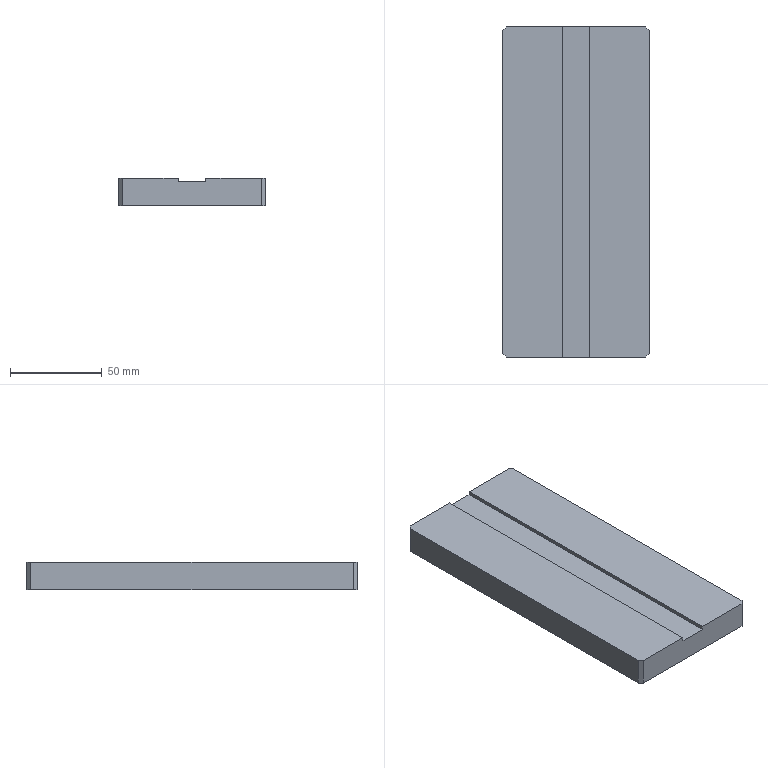Part | STEP file | Planar support platform base | 1 solid | 14 faces | box 80 x 180 x 15 mm | volume 210480 mm3 | plane 14
STEP:
#1=CARTESIAN_POINT('',(0.,0.,0.));
#2=DIRECTION('',(0.,0.,1.));
#3=DIRECTION('',(1.,0.,0.));
#4=AXIS2_PLACEMENT_3D('',#1,#2,#3);
#5=CARTESIAN_POINT('',(38.,90.,15.));
#6=VERTEX_POINT('',#5);
#7=CARTESIAN_POINT('',(7.5,90.,15.));
#8=VERTEX_POINT('',#7);
#9=CARTESIAN_POINT('',(-40.,90.,15.));
#10=DIRECTION('',(-1.,0.,0.));
#11=VECTOR('',#10,1.);
#12=LINE('',#9,#11);
#13=CARTESIAN_POINT('',(0.,0.,15.));
#14=DIRECTION('',(0.,0.,-1.));
#15=DIRECTION('',(-1.,0.,0.));
#16=AXIS2_PLACEMENT_3D('',#13,#14,#15);
#17=PLANE('',#16);
#18=CARTESIAN_POINT('',(40.,90.));
#19=DIRECTION('',(1.,0.));
#20=VECTOR('',#19,1.);
#21=LINE('',#18,#20);
#22=(GEOMETRIC_REPRESENTATION_CONTEXT(2)PARAMETRIC_REPRESENTATION_CONTEXT()REPRESENTATION_CONTEXT('',''));
#23=DEFINITIONAL_REPRESENTATION('',(#21),#22);
#24=PCURVE('',#17,#23);
#25=CARTESIAN_POINT('',(-40.,90.,15.));
#26=DIRECTION('',(0.,-1.,0.));
#27=DIRECTION('',(1.,0.,0.));
#28=AXIS2_PLACEMENT_3D('',#25,#26,#27);
#29=PLANE('',#28);
#30=CARTESIAN_POINT('',(0.,0.));
#31=DIRECTION('',(-1.,0.));
#32=VECTOR('',#31,1.);
#33=LINE('',#30,#32);
#34=(GEOMETRIC_REPRESENTATION_CONTEXT(2)PARAMETRIC_REPRESENTATION_CONTEXT()REPRESENTATION_CONTEXT('',''));
#35=DEFINITIONAL_REPRESENTATION('',(#33),#34);
#36=PCURVE('',#29,#35);
#37=SURFACE_CURVE('',#12,(#24,#36),.PCURVE_S1.);
#38=EDGE_CURVE('',#6,#8,#37,.T.);
#39=ORIENTED_EDGE('',*,*,#38,.T.);
#40=CARTESIAN_POINT('',(7.5,-90.,15.));
#41=VERTEX_POINT('',#40);
#42=CARTESIAN_POINT('',(7.5,-90.,15.));
#43=DIRECTION('',(0.,1.,0.));
#44=VECTOR('',#43,1.);
#45=LINE('',#42,#44);
#46=CARTESIAN_POINT('',(-7.5,-90.));
#47=DIRECTION('',(0.,1.));
#48=VECTOR('',#47,1.);
#49=LINE('',#46,#48);
#50=(GEOMETRIC_REPRESENTATION_CONTEXT(2)PARAMETRIC_REPRESENTATION_CONTEXT()REPRESENTATION_CONTEXT('',''));
#51=DEFINITIONAL_REPRESENTATION('',(#49),#50);
#52=PCURVE('',#17,#51);
#53=CARTESIAN_POINT('',(7.5,-90.,15.));
#54=DIRECTION('',(1.,0.,0.));
#55=DIRECTION('',(0.,0.,-1.));
#56=AXIS2_PLACEMENT_3D('',#53,#54,#55);
#57=PLANE('',#56);
#58=CARTESIAN_POINT('',(0.,0.));
#59=DIRECTION('',(0.,1.));
#60=VECTOR('',#59,1.);
#61=LINE('',#58,#60);
#62=(GEOMETRIC_REPRESENTATION_CONTEXT(2)PARAMETRIC_REPRESENTATION_CONTEXT()REPRESENTATION_CONTEXT('',''));
#63=DEFINITIONAL_REPRESENTATION('',(#61),#62);
#64=PCURVE('',#57,#63);
#65=SURFACE_CURVE('',#45,(#52,#64),.PCURVE_S1.);
#66=EDGE_CURVE('',#41,#8,#65,.T.);
#67=ORIENTED_EDGE('',*,*,#66,.F.);
#68=CARTESIAN_POINT('',(38.,-90.,15.));
#69=VERTEX_POINT('',#68);
#70=CARTESIAN_POINT('',(-40.,-90.,15.));
#71=DIRECTION('',(1.,0.,0.));
#72=VECTOR('',#71,1.);
#73=LINE('',#70,#72);
#74=CARTESIAN_POINT('',(40.,-90.));
#75=DIRECTION('',(-1.,0.));
#76=VECTOR('',#75,1.);
#77=LINE('',#74,#76);
#78=(GEOMETRIC_REPRESENTATION_CONTEXT(2)PARAMETRIC_REPRESENTATION_CONTEXT()REPRESENTATION_CONTEXT('',''));
#79=DEFINITIONAL_REPRESENTATION('',(#77),#78);
#80=PCURVE('',#17,#79);
#81=CARTESIAN_POINT('',(-40.,-90.,15.));
#82=DIRECTION('',(0.,1.,0.));
#83=DIRECTION('',(-1.,0.,0.));
#84=AXIS2_PLACEMENT_3D('',#81,#82,#83);
#85=PLANE('',#84);
#86=CARTESIAN_POINT('',(0.,0.));
#87=DIRECTION('',(-1.,0.));
#88=VECTOR('',#87,1.);
#89=LINE('',#86,#88);
#90=(GEOMETRIC_REPRESENTATION_CONTEXT(2)PARAMETRIC_REPRESENTATION_CONTEXT()REPRESENTATION_CONTEXT('',''));
#91=DEFINITIONAL_REPRESENTATION('',(#89),#90);
#92=PCURVE('',#85,#91);
#93=SURFACE_CURVE('',#73,(#80,#92),.PCURVE_S1.);
#94=EDGE_CURVE('',#41,#69,#93,.T.);
#95=ORIENTED_EDGE('',*,*,#94,.T.);
#96=CARTESIAN_POINT('',(40.,-88.,15.));
#97=VERTEX_POINT('',#96);
#98=CARTESIAN_POINT('',(40.,-88.,15.));
#99=DIRECTION('',(0.7071,0.7071,0.));
#100=VECTOR('',#99,1.);
#101=LINE('',#98,#100);
#102=CARTESIAN_POINT('',(-40.,-88.));
#103=DIRECTION('',(-0.7071,0.7071));
#104=VECTOR('',#103,1.);
#105=LINE('',#102,#104);
#106=(GEOMETRIC_REPRESENTATION_CONTEXT(2)PARAMETRIC_REPRESENTATION_CONTEXT()REPRESENTATION_CONTEXT('',''));
#107=DEFINITIONAL_REPRESENTATION('',(#105),#106);
#108=PCURVE('',#17,#107);
#109=CARTESIAN_POINT('',(40.,-88.,15.));
#110=DIRECTION('',(-0.7071,0.7071,0.));
#111=DIRECTION('',(0.,0.,-1.));
#112=AXIS2_PLACEMENT_3D('',#109,#110,#111);
#113=PLANE('',#112);
#114=CARTESIAN_POINT('',(0.,0.));
#115=DIRECTION('',(0.,-1.));
#116=VECTOR('',#115,1.);
#117=LINE('',#114,#116);
#118=(GEOMETRIC_REPRESENTATION_CONTEXT(2)PARAMETRIC_REPRESENTATION_CONTEXT()REPRESENTATION_CONTEXT('',''));
#119=DEFINITIONAL_REPRESENTATION('',(#117),#118);
#120=PCURVE('',#113,#119);
#121=SURFACE_CURVE('',#101,(#108,#120),.PCURVE_S1.);
#122=EDGE_CURVE('',#69,#97,#121,.T.);
#123=ORIENTED_EDGE('',*,*,#122,.T.);
#124=CARTESIAN_POINT('',(40.,88.,15.));
#125=VERTEX_POINT('',#124);
#126=CARTESIAN_POINT('',(40.,-90.,15.));
#127=DIRECTION('',(0.,1.,0.));
#128=VECTOR('',#127,1.);
#129=LINE('',#126,#128);
#130=CARTESIAN_POINT('',(-40.,-90.));
#131=DIRECTION('',(0.,1.));
#132=VECTOR('',#131,1.);
#133=LINE('',#130,#132);
#134=(GEOMETRIC_REPRESENTATION_CONTEXT(2)PARAMETRIC_REPRESENTATION_CONTEXT()REPRESENTATION_CONTEXT('',''));
#135=DEFINITIONAL_REPRESENTATION('',(#133),#134);
#136=PCURVE('',#17,#135);
#137=CARTESIAN_POINT('',(40.,-90.,15.));
#138=DIRECTION('',(-1.,0.,0.));
#139=DIRECTION('',(0.,0.,1.));
#140=AXIS2_PLACEMENT_3D('',#137,#138,#139);
#141=PLANE('',#140);
#142=CARTESIAN_POINT('',(0.,0.));
#143=DIRECTION('',(0.,1.));
#144=VECTOR('',#143,1.);
#145=LINE('',#142,#144);
#146=(GEOMETRIC_REPRESENTATION_CONTEXT(2)PARAMETRIC_REPRESENTATION_CONTEXT()REPRESENTATION_CONTEXT('',''));
#147=DEFINITIONAL_REPRESENTATION('',(#145),#146);
#148=PCURVE('',#141,#147);
#149=SURFACE_CURVE('',#129,(#136,#148),.PCURVE_S1.);
#150=EDGE_CURVE('',#97,#125,#149,.T.);
#151=ORIENTED_EDGE('',*,*,#150,.T.);
#152=CARTESIAN_POINT('',(38.,90.,15.));
#153=DIRECTION('',(-0.7071,0.7071,0.));
#154=VECTOR('',#153,1.);
#155=LINE('',#152,#154);
#156=CARTESIAN_POINT('',(-38.,90.));
#157=DIRECTION('',(0.7071,0.7071));
#158=VECTOR('',#157,1.);
#159=LINE('',#156,#158);
#160=(GEOMETRIC_REPRESENTATION_CONTEXT(2)PARAMETRIC_REPRESENTATION_CONTEXT()REPRESENTATION_CONTEXT('',''));
#161=DEFINITIONAL_REPRESENTATION('',(#159),#160);
#162=PCURVE('',#17,#161);
#163=CARTESIAN_POINT('',(38.,90.,15.));
#164=DIRECTION('',(-0.7071,-0.7071,0.));
#165=DIRECTION('',(0.,0.,-1.));
#166=AXIS2_PLACEMENT_3D('',#163,#164,#165);
#167=PLANE('',#166);
#168=CARTESIAN_POINT('',(0.,0.));
#169=DIRECTION('',(0.,-1.));
#170=VECTOR('',#169,1.);
#171=LINE('',#168,#170);
#172=(GEOMETRIC_REPRESENTATION_CONTEXT(2)PARAMETRIC_REPRESENTATION_CONTEXT()REPRESENTATION_CONTEXT('',''));
#173=DEFINITIONAL_REPRESENTATION('',(#171),#172);
#174=PCURVE('',#167,#173);
#175=SURFACE_CURVE('',#155,(#162,#174),.PCURVE_S1.);
#176=EDGE_CURVE('',#125,#6,#175,.T.);
#177=ORIENTED_EDGE('',*,*,#176,.T.);
#178=EDGE_LOOP('',(#39,#67,#95,#123,#151,#177));
#179=FACE_BOUND('',#178,.T.);
#180=ADVANCED_FACE('',(#179),#17,.F.);
#181=ORIENTED_EDGE('',*,*,#150,.F.);
#182=CARTESIAN_POINT('',(40.,-88.,0.));
#183=VERTEX_POINT('',#182);
#184=CARTESIAN_POINT('',(40.,-88.,15.));
#185=DIRECTION('',(0.,0.,-1.));
#186=VECTOR('',#185,1.);
#187=LINE('',#184,#186);
#188=CARTESIAN_POINT('',(0.,2.));
#189=DIRECTION('',(-1.,0.));
#190=VECTOR('',#189,1.);
#191=LINE('',#188,#190);
#192=(GEOMETRIC_REPRESENTATION_CONTEXT(2)PARAMETRIC_REPRESENTATION_CONTEXT()REPRESENTATION_CONTEXT('',''));
#193=DEFINITIONAL_REPRESENTATION('',(#191),#192);
#194=PCURVE('',#141,#193);
#195=CARTESIAN_POINT('',(0.,0.));
#196=DIRECTION('',(1.,0.));
#197=VECTOR('',#196,1.);
#198=LINE('',#195,#197);
#199=(GEOMETRIC_REPRESENTATION_CONTEXT(2)PARAMETRIC_REPRESENTATION_CONTEXT()REPRESENTATION_CONTEXT('',''));
#200=DEFINITIONAL_REPRESENTATION('',(#198),#199);
#201=PCURVE('',#113,#200);
#202=SURFACE_CURVE('',#187,(#194,#201),.PCURVE_S1.);
#203=EDGE_CURVE('',#97,#183,#202,.T.);
#204=ORIENTED_EDGE('',*,*,#203,.T.);
#205=CARTESIAN_POINT('',(40.,88.,0.));
#206=VERTEX_POINT('',#205);
#207=CARTESIAN_POINT('',(40.,-90.,0.));
#208=DIRECTION('',(0.,1.,0.));
#209=VECTOR('',#208,1.);
#210=LINE('',#207,#209);
#211=CARTESIAN_POINT('',(-15.,0.));
#212=DIRECTION('',(0.,1.));
#213=VECTOR('',#212,1.);
#214=LINE('',#211,#213);
#215=(GEOMETRIC_REPRESENTATION_CONTEXT(2)PARAMETRIC_REPRESENTATION_CONTEXT()REPRESENTATION_CONTEXT('',''));
#216=DEFINITIONAL_REPRESENTATION('',(#214),#215);
#217=PCURVE('',#141,#216);
#218=CARTESIAN_POINT('',(0.,0.,0.));
#219=DIRECTION('',(0.,0.,-1.));
#220=DIRECTION('',(-1.,0.,0.));
#221=AXIS2_PLACEMENT_3D('',#218,#219,#220);
#222=PLANE('',#221);
#223=CARTESIAN_POINT('',(-40.,-90.));
#224=DIRECTION('',(0.,1.));
#225=VECTOR('',#224,1.);
#226=LINE('',#223,#225);
#227=(GEOMETRIC_REPRESENTATION_CONTEXT(2)PARAMETRIC_REPRESENTATION_CONTEXT()REPRESENTATION_CONTEXT('',''));
#228=DEFINITIONAL_REPRESENTATION('',(#226),#227);
#229=PCURVE('',#222,#228);
#230=SURFACE_CURVE('',#210,(#217,#229),.PCURVE_S1.);
#231=EDGE_CURVE('',#183,#206,#230,.T.);
#232=ORIENTED_EDGE('',*,*,#231,.T.);
#233=CARTESIAN_POINT('',(40.,88.,15.));
#234=DIRECTION('',(0.,0.,1.));
#235=VECTOR('',#234,1.);
#236=LINE('',#233,#235);
#237=CARTESIAN_POINT('',(0.,178.));
#238=DIRECTION('',(1.,0.));
#239=VECTOR('',#238,1.);
#240=LINE('',#237,#239);
#241=(GEOMETRIC_REPRESENTATION_CONTEXT(2)PARAMETRIC_REPRESENTATION_CONTEXT()REPRESENTATION_CONTEXT('',''));
#242=DEFINITIONAL_REPRESENTATION('',(#240),#241);
#243=PCURVE('',#141,#242);
#244=CARTESIAN_POINT('',(0.,2.828));
#245=DIRECTION('',(-1.,0.));
#246=VECTOR('',#245,1.);
#247=LINE('',#244,#246);
#248=(GEOMETRIC_REPRESENTATION_CONTEXT(2)PARAMETRIC_REPRESENTATION_CONTEXT()REPRESENTATION_CONTEXT('',''));
#249=DEFINITIONAL_REPRESENTATION('',(#247),#248);
#250=PCURVE('',#167,#249);
#251=SURFACE_CURVE('',#236,(#243,#250),.PCURVE_S1.);
#252=EDGE_CURVE('',#206,#125,#251,.T.);
#253=ORIENTED_EDGE('',*,*,#252,.T.);
#254=EDGE_LOOP('',(#181,#204,#232,#253));
#255=FACE_BOUND('',#254,.T.);
#256=ADVANCED_FACE('',(#255),#141,.F.);
#257=CARTESIAN_POINT('',(7.5,90.,13.));
#258=VERTEX_POINT('',#257);
#259=CARTESIAN_POINT('',(-7.5,90.,13.));
#260=VERTEX_POINT('',#259);
#261=CARTESIAN_POINT('',(7.5,90.,13.));
#262=DIRECTION('',(-1.,0.,0.));
#263=VECTOR('',#262,1.);
#264=LINE('',#261,#263);
#265=CARTESIAN_POINT('',(47.5,-2.));
#266=DIRECTION('',(-1.,0.));
#267=VECTOR('',#266,1.);
#268=LINE('',#265,#267);
#269=(GEOMETRIC_REPRESENTATION_CONTEXT(2)PARAMETRIC_REPRESENTATION_CONTEXT()REPRESENTATION_CONTEXT('',''));
#270=DEFINITIONAL_REPRESENTATION('',(#268),#269);
#271=PCURVE('',#29,#270);
#272=CARTESIAN_POINT('',(7.5,-90.,13.));
#273=DIRECTION('',(0.,0.,-1.));
#274=DIRECTION('',(-1.,0.,0.));
#275=AXIS2_PLACEMENT_3D('',#272,#273,#274);
#276=PLANE('',#275);
#277=CARTESIAN_POINT('',(0.,180.));
#278=DIRECTION('',(1.,0.));
#279=VECTOR('',#278,1.);
#280=LINE('',#277,#279);
#281=(GEOMETRIC_REPRESENTATION_CONTEXT(2)PARAMETRIC_REPRESENTATION_CONTEXT()REPRESENTATION_CONTEXT('',''));
#282=DEFINITIONAL_REPRESENTATION('',(#280),#281);
#283=PCURVE('',#276,#282);
#284=SURFACE_CURVE('',#264,(#271,#283),.PCURVE_S1.);
#285=EDGE_CURVE('',#258,#260,#284,.T.);
#286=ORIENTED_EDGE('',*,*,#285,.F.);
#287=CARTESIAN_POINT('',(7.5,90.,15.));
#288=DIRECTION('',(0.,0.,-1.));
#289=VECTOR('',#288,1.);
#290=LINE('',#287,#289);
#291=CARTESIAN_POINT('',(47.5,0.));
#292=DIRECTION('',(0.,-1.));
#293=VECTOR('',#292,1.);
#294=LINE('',#291,#293);
#295=(GEOMETRIC_REPRESENTATION_CONTEXT(2)PARAMETRIC_REPRESENTATION_CONTEXT()REPRESENTATION_CONTEXT('',''));
#296=DEFINITIONAL_REPRESENTATION('',(#294),#295);
#297=PCURVE('',#29,#296);
#298=CARTESIAN_POINT('',(0.,180.));
#299=DIRECTION('',(1.,0.));
#300=VECTOR('',#299,1.);
#301=LINE('',#298,#300);
#302=(GEOMETRIC_REPRESENTATION_CONTEXT(2)PARAMETRIC_REPRESENTATION_CONTEXT()REPRESENTATION_CONTEXT('',''));
#303=DEFINITIONAL_REPRESENTATION('',(#301),#302);
#304=PCURVE('',#57,#303);
#305=SURFACE_CURVE('',#290,(#297,#304),.PCURVE_S1.);
#306=EDGE_CURVE('',#8,#258,#305,.T.);
#307=ORIENTED_EDGE('',*,*,#306,.F.);
#308=ORIENTED_EDGE('',*,*,#38,.F.);
#309=CARTESIAN_POINT('',(38.,90.,0.));
#310=VERTEX_POINT('',#309);
#311=CARTESIAN_POINT('',(38.,90.,15.));
#312=DIRECTION('',(0.,0.,-1.));
#313=VECTOR('',#312,1.);
#314=LINE('',#311,#313);
#315=CARTESIAN_POINT('',(78.,0.));
#316=DIRECTION('',(0.,-1.));
#317=VECTOR('',#316,1.);
#318=LINE('',#315,#317);
#319=(GEOMETRIC_REPRESENTATION_CONTEXT(2)PARAMETRIC_REPRESENTATION_CONTEXT()REPRESENTATION_CONTEXT('',''));
#320=DEFINITIONAL_REPRESENTATION('',(#318),#319);
#321=PCURVE('',#29,#320);
#322=CARTESIAN_POINT('',(0.,0.));
#323=DIRECTION('',(1.,0.));
#324=VECTOR('',#323,1.);
#325=LINE('',#322,#324);
#326=(GEOMETRIC_REPRESENTATION_CONTEXT(2)PARAMETRIC_REPRESENTATION_CONTEXT()REPRESENTATION_CONTEXT('',''));
#327=DEFINITIONAL_REPRESENTATION('',(#325),#326);
#328=PCURVE('',#167,#327);
#329=SURFACE_CURVE('',#314,(#321,#328),.PCURVE_S1.);
#330=EDGE_CURVE('',#6,#310,#329,.T.);
#331=ORIENTED_EDGE('',*,*,#330,.T.);
#332=CARTESIAN_POINT('',(-38.,90.,0.));
#333=VERTEX_POINT('',#332);
#334=CARTESIAN_POINT('',(-40.,90.,0.));
#335=DIRECTION('',(-1.,0.,0.));
#336=VECTOR('',#335,1.);
#337=LINE('',#334,#336);
#338=CARTESIAN_POINT('',(0.,-15.));
#339=DIRECTION('',(-1.,0.));
#340=VECTOR('',#339,1.);
#341=LINE('',#338,#340);
#342=(GEOMETRIC_REPRESENTATION_CONTEXT(2)PARAMETRIC_REPRESENTATION_CONTEXT()REPRESENTATION_CONTEXT('',''));
#343=DEFINITIONAL_REPRESENTATION('',(#341),#342);
#344=PCURVE('',#29,#343);
#345=CARTESIAN_POINT('',(40.,90.));
#346=DIRECTION('',(1.,0.));
#347=VECTOR('',#346,1.);
#348=LINE('',#345,#347);
#349=(GEOMETRIC_REPRESENTATION_CONTEXT(2)PARAMETRIC_REPRESENTATION_CONTEXT()REPRESENTATION_CONTEXT('',''));
#350=DEFINITIONAL_REPRESENTATION('',(#348),#349);
#351=PCURVE('',#222,#350);
#352=SURFACE_CURVE('',#337,(#344,#351),.PCURVE_S1.);
#353=EDGE_CURVE('',#310,#333,#352,.T.);
#354=ORIENTED_EDGE('',*,*,#353,.T.);
#355=CARTESIAN_POINT('',(-38.,90.,15.));
#356=VERTEX_POINT('',#355);
#357=CARTESIAN_POINT('',(-38.,90.,15.));
#358=DIRECTION('',(0.,0.,1.));
#359=VECTOR('',#358,1.);
#360=LINE('',#357,#359);
#361=CARTESIAN_POINT('',(2.,0.));
#362=DIRECTION('',(0.,1.));
#363=VECTOR('',#362,1.);
#364=LINE('',#361,#363);
#365=(GEOMETRIC_REPRESENTATION_CONTEXT(2)PARAMETRIC_REPRESENTATION_CONTEXT()REPRESENTATION_CONTEXT('',''));
#366=DEFINITIONAL_REPRESENTATION('',(#364),#365);
#367=PCURVE('',#29,#366);
#368=CARTESIAN_POINT('',(-40.,88.,15.));
#369=DIRECTION('',(0.7071,-0.7071,0.));
#370=DIRECTION('',(0.,0.,-1.));
#371=AXIS2_PLACEMENT_3D('',#368,#369,#370);
#372=PLANE('',#371);
#373=CARTESIAN_POINT('',(0.,2.828));
#374=DIRECTION('',(-1.,0.));
#375=VECTOR('',#374,1.);
#376=LINE('',#373,#375);
#377=(GEOMETRIC_REPRESENTATION_CONTEXT(2)PARAMETRIC_REPRESENTATION_CONTEXT()REPRESENTATION_CONTEXT('',''));
#378=DEFINITIONAL_REPRESENTATION('',(#376),#377);
#379=PCURVE('',#372,#378);
#380=SURFACE_CURVE('',#360,(#367,#379),.PCURVE_S1.);
#381=EDGE_CURVE('',#333,#356,#380,.T.);
#382=ORIENTED_EDGE('',*,*,#381,.T.);
#383=CARTESIAN_POINT('',(-7.5,90.,15.));
#384=VERTEX_POINT('',#383);
#385=CARTESIAN_POINT('',(-40.,90.,15.));
#386=DIRECTION('',(-1.,0.,0.));
#387=VECTOR('',#386,1.);
#388=LINE('',#385,#387);
#389=CARTESIAN_POINT('',(0.,0.));
#390=DIRECTION('',(-1.,0.));
#391=VECTOR('',#390,1.);
#392=LINE('',#389,#391);
#393=(GEOMETRIC_REPRESENTATION_CONTEXT(2)PARAMETRIC_REPRESENTATION_CONTEXT()REPRESENTATION_CONTEXT('',''));
#394=DEFINITIONAL_REPRESENTATION('',(#392),#393);
#395=PCURVE('',#29,#394);
#396=CARTESIAN_POINT('',(0.,0.,15.));
#397=DIRECTION('',(0.,0.,-1.));
#398=DIRECTION('',(-1.,0.,0.));
#399=AXIS2_PLACEMENT_3D('',#396,#397,#398);
#400=PLANE('',#399);
#401=CARTESIAN_POINT('',(40.,90.));
#402=DIRECTION('',(1.,0.));
#403=VECTOR('',#402,1.);
#404=LINE('',#401,#403);
#405=(GEOMETRIC_REPRESENTATION_CONTEXT(2)PARAMETRIC_REPRESENTATION_CONTEXT()REPRESENTATION_CONTEXT('',''));
#406=DEFINITIONAL_REPRESENTATION('',(#404),#405);
#407=PCURVE('',#400,#406);
#408=SURFACE_CURVE('',#388,(#395,#407),.PCURVE_S1.);
#409=EDGE_CURVE('',#384,#356,#408,.T.);
#410=ORIENTED_EDGE('',*,*,#409,.F.);
#411=CARTESIAN_POINT('',(-7.5,90.,15.));
#412=DIRECTION('',(0.,0.,1.));
#413=VECTOR('',#412,1.);
#414=LINE('',#411,#413);
#415=CARTESIAN_POINT('',(32.5,0.));
#416=DIRECTION('',(0.,1.));
#417=VECTOR('',#416,1.);
#418=LINE('',#415,#417);
#419=(GEOMETRIC_REPRESENTATION_CONTEXT(2)PARAMETRIC_REPRESENTATION_CONTEXT()REPRESENTATION_CONTEXT('',''));
#420=DEFINITIONAL_REPRESENTATION('',(#418),#419);
#421=PCURVE('',#29,#420);
#422=CARTESIAN_POINT('',(-7.5,-90.,15.));
#423=DIRECTION('',(-1.,0.,0.));
#424=DIRECTION('',(0.,-1.,0.));
#425=AXIS2_PLACEMENT_3D('',#422,#423,#424);
#426=PLANE('',#425);
#427=CARTESIAN_POINT('',(-180.,0.));
#428=DIRECTION('',(0.,1.));
#429=VECTOR('',#428,1.);
#430=LINE('',#427,#429);
#431=(GEOMETRIC_REPRESENTATION_CONTEXT(2)PARAMETRIC_REPRESENTATION_CONTEXT()REPRESENTATION_CONTEXT('',''));
#432=DEFINITIONAL_REPRESENTATION('',(#430),#431);
#433=PCURVE('',#426,#432);
#434=SURFACE_CURVE('',#414,(#421,#433),.PCURVE_S1.);
#435=EDGE_CURVE('',#260,#384,#434,.T.);
#436=ORIENTED_EDGE('',*,*,#435,.F.);
#437=EDGE_LOOP('',(#286,#307,#308,#331,#354,#382,#410,#436));
#438=FACE_BOUND('',#437,.T.);
#439=ADVANCED_FACE('',(#438),#29,.F.);
#440=CARTESIAN_POINT('',(-40.,88.,0.));
#441=VERTEX_POINT('',#440);
#442=CARTESIAN_POINT('',(-40.,-88.,0.));
#443=VERTEX_POINT('',#442);
#444=CARTESIAN_POINT('',(-40.,-90.,0.));
#445=DIRECTION('',(0.,-1.,0.));
#446=VECTOR('',#445,1.);
#447=LINE('',#444,#446);
#448=CARTESIAN_POINT('',(-40.,-90.,15.));
#449=DIRECTION('',(1.,0.,0.));
#450=DIRECTION('',(0.,1.,0.));
#451=AXIS2_PLACEMENT_3D('',#448,#449,#450);
#452=PLANE('',#451);
#453=CARTESIAN_POINT('',(0.,-15.));
#454=DIRECTION('',(-1.,0.));
#455=VECTOR('',#454,1.);
#456=LINE('',#453,#455);
#457=(GEOMETRIC_REPRESENTATION_CONTEXT(2)PARAMETRIC_REPRESENTATION_CONTEXT()REPRESENTATION_CONTEXT('',''));
#458=DEFINITIONAL_REPRESENTATION('',(#456),#457);
#459=PCURVE('',#452,#458);
#460=CARTESIAN_POINT('',(40.,-90.));
#461=DIRECTION('',(0.,-1.));
#462=VECTOR('',#461,1.);
#463=LINE('',#460,#462);
#464=(GEOMETRIC_REPRESENTATION_CONTEXT(2)PARAMETRIC_REPRESENTATION_CONTEXT()REPRESENTATION_CONTEXT('',''));
#465=DEFINITIONAL_REPRESENTATION('',(#463),#464);
#466=PCURVE('',#222,#465);
#467=SURFACE_CURVE('',#447,(#459,#466),.PCURVE_S1.);
#468=EDGE_CURVE('',#441,#443,#467,.T.);
#469=ORIENTED_EDGE('',*,*,#468,.T.);
#470=CARTESIAN_POINT('',(-40.,-88.,15.));
#471=VERTEX_POINT('',#470);
#472=CARTESIAN_POINT('',(-40.,-88.,15.));
#473=DIRECTION('',(0.,0.,1.));
#474=VECTOR('',#473,1.);
#475=LINE('',#472,#474);
#476=CARTESIAN_POINT('',(2.,0.));
#477=DIRECTION('',(0.,1.));
#478=VECTOR('',#477,1.);
#479=LINE('',#476,#478);
#480=(GEOMETRIC_REPRESENTATION_CONTEXT(2)PARAMETRIC_REPRESENTATION_CONTEXT()REPRESENTATION_CONTEXT('',''));
#481=DEFINITIONAL_REPRESENTATION('',(#479),#480);
#482=PCURVE('',#452,#481);
#483=CARTESIAN_POINT('',(-38.,-90.,15.));
#484=DIRECTION('',(0.7071,0.7071,0.));
#485=DIRECTION('',(0.,0.,-1.));
#486=AXIS2_PLACEMENT_3D('',#483,#484,#485);
#487=PLANE('',#486);
#488=CARTESIAN_POINT('',(0.,2.828));
#489=DIRECTION('',(-1.,0.));
#490=VECTOR('',#489,1.);
#491=LINE('',#488,#490);
#492=(GEOMETRIC_REPRESENTATION_CONTEXT(2)PARAMETRIC_REPRESENTATION_CONTEXT()REPRESENTATION_CONTEXT('',''));
#493=DEFINITIONAL_REPRESENTATION('',(#491),#492);
#494=PCURVE('',#487,#493);
#495=SURFACE_CURVE('',#475,(#482,#494),.PCURVE_S1.);
#496=EDGE_CURVE('',#443,#471,#495,.T.);
#497=ORIENTED_EDGE('',*,*,#496,.T.);
#498=CARTESIAN_POINT('',(-40.,88.,15.));
#499=VERTEX_POINT('',#498);
#500=CARTESIAN_POINT('',(-40.,-90.,15.));
#501=DIRECTION('',(0.,-1.,0.));
#502=VECTOR('',#501,1.);
#503=LINE('',#500,#502);
#504=CARTESIAN_POINT('',(0.,0.));
#505=DIRECTION('',(-1.,0.));
#506=VECTOR('',#505,1.);
#507=LINE('',#504,#506);
#508=(GEOMETRIC_REPRESENTATION_CONTEXT(2)PARAMETRIC_REPRESENTATION_CONTEXT()REPRESENTATION_CONTEXT('',''));
#509=DEFINITIONAL_REPRESENTATION('',(#507),#508);
#510=PCURVE('',#452,#509);
#511=CARTESIAN_POINT('',(40.,-90.));
#512=DIRECTION('',(0.,-1.));
#513=VECTOR('',#512,1.);
#514=LINE('',#511,#513);
#515=(GEOMETRIC_REPRESENTATION_CONTEXT(2)PARAMETRIC_REPRESENTATION_CONTEXT()REPRESENTATION_CONTEXT('',''));
#516=DEFINITIONAL_REPRESENTATION('',(#514),#515);
#517=PCURVE('',#400,#516);
#518=SURFACE_CURVE('',#503,(#510,#517),.PCURVE_S1.);
#519=EDGE_CURVE('',#499,#471,#518,.T.);
#520=ORIENTED_EDGE('',*,*,#519,.F.);
#521=CARTESIAN_POINT('',(-40.,88.,15.));
#522=DIRECTION('',(0.,0.,-1.));
#523=VECTOR('',#522,1.);
#524=LINE('',#521,#523);
#525=CARTESIAN_POINT('',(178.,0.));
#526=DIRECTION('',(0.,-1.));
#527=VECTOR('',#526,1.);
#528=LINE('',#525,#527);
#529=(GEOMETRIC_REPRESENTATION_CONTEXT(2)PARAMETRIC_REPRESENTATION_CONTEXT()REPRESENTATION_CONTEXT('',''));
#530=DEFINITIONAL_REPRESENTATION('',(#528),#529);
#531=PCURVE('',#452,#530);
#532=CARTESIAN_POINT('',(0.,0.));
#533=DIRECTION('',(1.,0.));
#534=VECTOR('',#533,1.);
#535=LINE('',#532,#534);
#536=(GEOMETRIC_REPRESENTATION_CONTEXT(2)PARAMETRIC_REPRESENTATION_CONTEXT()REPRESENTATION_CONTEXT('',''));
#537=DEFINITIONAL_REPRESENTATION('',(#535),#536);
#538=PCURVE('',#372,#537);
#539=SURFACE_CURVE('',#524,(#531,#538),.PCURVE_S1.);
#540=EDGE_CURVE('',#499,#441,#539,.T.);
#541=ORIENTED_EDGE('',*,*,#540,.T.);
#542=EDGE_LOOP('',(#469,#497,#520,#541));
#543=FACE_BOUND('',#542,.T.);
#544=ADVANCED_FACE('',(#543),#452,.F.);
#545=ORIENTED_EDGE('',*,*,#94,.F.);
#546=CARTESIAN_POINT('',(7.5,-90.,13.));
#547=VERTEX_POINT('',#546);
#548=CARTESIAN_POINT('',(7.5,-90.,15.));
#549=DIRECTION('',(0.,0.,-1.));
#550=VECTOR('',#549,1.);
#551=LINE('',#548,#550);
#552=CARTESIAN_POINT('',(-47.5,0.));
#553=DIRECTION('',(0.,-1.));
#554=VECTOR('',#553,1.);
#555=LINE('',#552,#554);
#556=(GEOMETRIC_REPRESENTATION_CONTEXT(2)PARAMETRIC_REPRESENTATION_CONTEXT()REPRESENTATION_CONTEXT('',''));
#557=DEFINITIONAL_REPRESENTATION('',(#555),#556);
#558=PCURVE('',#85,#557);
#559=CARTESIAN_POINT('',(0.,0.));
#560=DIRECTION('',(1.,0.));
#561=VECTOR('',#560,1.);
#562=LINE('',#559,#561);
#563=(GEOMETRIC_REPRESENTATION_CONTEXT(2)PARAMETRIC_REPRESENTATION_CONTEXT()REPRESENTATION_CONTEXT('',''));
#564=DEFINITIONAL_REPRESENTATION('',(#562),#563);
#565=PCURVE('',#57,#564);
#566=SURFACE_CURVE('',#551,(#558,#565),.PCURVE_S1.);
#567=EDGE_CURVE('',#41,#547,#566,.T.);
#568=ORIENTED_EDGE('',*,*,#567,.T.);
#569=CARTESIAN_POINT('',(-7.5,-90.,13.));
#570=VERTEX_POINT('',#569);
#571=CARTESIAN_POINT('',(7.5,-90.,13.));
#572=DIRECTION('',(-1.,0.,0.));
#573=VECTOR('',#572,1.);
#574=LINE('',#571,#573);
#575=CARTESIAN_POINT('',(-47.5,-2.));
#576=DIRECTION('',(1.,0.));
#577=VECTOR('',#576,1.);
#578=LINE('',#575,#577);
#579=(GEOMETRIC_REPRESENTATION_CONTEXT(2)PARAMETRIC_REPRESENTATION_CONTEXT()REPRESENTATION_CONTEXT('',''));
#580=DEFINITIONAL_REPRESENTATION('',(#578),#579);
#581=PCURVE('',#85,#580);
#582=CARTESIAN_POINT('',(0.,0.));
#583=DIRECTION('',(1.,0.));
#584=VECTOR('',#583,1.);
#585=LINE('',#582,#584);
#586=(GEOMETRIC_REPRESENTATION_CONTEXT(2)PARAMETRIC_REPRESENTATION_CONTEXT()REPRESENTATION_CONTEXT('',''));
#587=DEFINITIONAL_REPRESENTATION('',(#585),#586);
#588=PCURVE('',#276,#587);
#589=SURFACE_CURVE('',#574,(#581,#588),.PCURVE_S1.);
#590=EDGE_CURVE('',#547,#570,#589,.T.);
#591=ORIENTED_EDGE('',*,*,#590,.T.);
#592=CARTESIAN_POINT('',(-7.5,-90.,15.));
#593=VERTEX_POINT('',#592);
#594=CARTESIAN_POINT('',(-7.5,-90.,15.));
#595=DIRECTION('',(0.,0.,1.));
#596=VECTOR('',#595,1.);
#597=LINE('',#594,#596);
#598=CARTESIAN_POINT('',(-32.5,0.));
#599=DIRECTION('',(0.,1.));
#600=VECTOR('',#599,1.);
#601=LINE('',#598,#600);
#602=(GEOMETRIC_REPRESENTATION_CONTEXT(2)PARAMETRIC_REPRESENTATION_CONTEXT()REPRESENTATION_CONTEXT('',''));
#603=DEFINITIONAL_REPRESENTATION('',(#601),#602);
#604=PCURVE('',#85,#603);
#605=CARTESIAN_POINT('',(0.,0.));
#606=DIRECTION('',(0.,1.));
#607=VECTOR('',#606,1.);
#608=LINE('',#605,#607);
#609=(GEOMETRIC_REPRESENTATION_CONTEXT(2)PARAMETRIC_REPRESENTATION_CONTEXT()REPRESENTATION_CONTEXT('',''));
#610=DEFINITIONAL_REPRESENTATION('',(#608),#609);
#611=PCURVE('',#426,#610);
#612=SURFACE_CURVE('',#597,(#604,#611),.PCURVE_S1.);
#613=EDGE_CURVE('',#570,#593,#612,.T.);
#614=ORIENTED_EDGE('',*,*,#613,.T.);
#615=CARTESIAN_POINT('',(-38.,-90.,15.));
#616=VERTEX_POINT('',#615);
#617=CARTESIAN_POINT('',(-40.,-90.,15.));
#618=DIRECTION('',(1.,0.,0.));
#619=VECTOR('',#618,1.);
#620=LINE('',#617,#619);
#621=CARTESIAN_POINT('',(0.,0.));
#622=DIRECTION('',(-1.,0.));
#623=VECTOR('',#622,1.);
#624=LINE('',#621,#623);
#625=(GEOMETRIC_REPRESENTATION_CONTEXT(2)PARAMETRIC_REPRESENTATION_CONTEXT()REPRESENTATION_CONTEXT('',''));
#626=DEFINITIONAL_REPRESENTATION('',(#624),#625);
#627=PCURVE('',#85,#626);
#628=CARTESIAN_POINT('',(40.,-90.));
#629=DIRECTION('',(-1.,0.));
#630=VECTOR('',#629,1.);
#631=LINE('',#628,#630);
#632=(GEOMETRIC_REPRESENTATION_CONTEXT(2)PARAMETRIC_REPRESENTATION_CONTEXT()REPRESENTATION_CONTEXT('',''));
#633=DEFINITIONAL_REPRESENTATION('',(#631),#632);
#634=PCURVE('',#400,#633);
#635=SURFACE_CURVE('',#620,(#627,#634),.PCURVE_S1.);
#636=EDGE_CURVE('',#616,#593,#635,.T.);
#637=ORIENTED_EDGE('',*,*,#636,.F.);
#638=CARTESIAN_POINT('',(-38.,-90.,0.));
#639=VERTEX_POINT('',#638);
#640=CARTESIAN_POINT('',(-38.,-90.,15.));
#641=DIRECTION('',(0.,0.,-1.));
#642=VECTOR('',#641,1.);
#643=LINE('',#640,#642);
#644=CARTESIAN_POINT('',(-2.,0.));
#645=DIRECTION('',(0.,-1.));
#646=VECTOR('',#645,1.);
#647=LINE('',#644,#646);
#648=(GEOMETRIC_REPRESENTATION_CONTEXT(2)PARAMETRIC_REPRESENTATION_CONTEXT()REPRESENTATION_CONTEXT('',''));
#649=DEFINITIONAL_REPRESENTATION('',(#647),#648);
#650=PCURVE('',#85,#649);
#651=CARTESIAN_POINT('',(0.,0.));
#652=DIRECTION('',(1.,0.));
#653=VECTOR('',#652,1.);
#654=LINE('',#651,#653);
#655=(GEOMETRIC_REPRESENTATION_CONTEXT(2)PARAMETRIC_REPRESENTATION_CONTEXT()REPRESENTATION_CONTEXT('',''));
#656=DEFINITIONAL_REPRESENTATION('',(#654),#655);
#657=PCURVE('',#487,#656);
#658=SURFACE_CURVE('',#643,(#650,#657),.PCURVE_S1.);
#659=EDGE_CURVE('',#616,#639,#658,.T.);
#660=ORIENTED_EDGE('',*,*,#659,.T.);
#661=CARTESIAN_POINT('',(38.,-90.,0.));
#662=VERTEX_POINT('',#661);
#663=CARTESIAN_POINT('',(-40.,-90.,0.));
#664=DIRECTION('',(1.,0.,0.));
#665=VECTOR('',#664,1.);
#666=LINE('',#663,#665);
#667=CARTESIAN_POINT('',(0.,-15.));
#668=DIRECTION('',(-1.,0.));
#669=VECTOR('',#668,1.);
#670=LINE('',#667,#669);
#671=(GEOMETRIC_REPRESENTATION_CONTEXT(2)PARAMETRIC_REPRESENTATION_CONTEXT()REPRESENTATION_CONTEXT('',''));
#672=DEFINITIONAL_REPRESENTATION('',(#670),#671);
#673=PCURVE('',#85,#672);
#674=CARTESIAN_POINT('',(40.,-90.));
#675=DIRECTION('',(-1.,0.));
#676=VECTOR('',#675,1.);
#677=LINE('',#674,#676);
#678=(GEOMETRIC_REPRESENTATION_CONTEXT(2)PARAMETRIC_REPRESENTATION_CONTEXT()REPRESENTATION_CONTEXT('',''));
#679=DEFINITIONAL_REPRESENTATION('',(#677),#678);
#680=PCURVE('',#222,#679);
#681=SURFACE_CURVE('',#666,(#673,#680),.PCURVE_S1.);
#682=EDGE_CURVE('',#639,#662,#681,.T.);
#683=ORIENTED_EDGE('',*,*,#682,.T.);
#684=CARTESIAN_POINT('',(38.,-90.,15.));
#685=DIRECTION('',(0.,0.,1.));
#686=VECTOR('',#685,1.);
#687=LINE('',#684,#686);
#688=CARTESIAN_POINT('',(-78.,0.));
#689=DIRECTION('',(0.,1.));
#690=VECTOR('',#689,1.);
#691=LINE('',#688,#690);
#692=(GEOMETRIC_REPRESENTATION_CONTEXT(2)PARAMETRIC_REPRESENTATION_CONTEXT()REPRESENTATION_CONTEXT('',''));
#693=DEFINITIONAL_REPRESENTATION('',(#691),#692);
#694=PCURVE('',#85,#693);
#695=CARTESIAN_POINT('',(0.,2.828));
#696=DIRECTION('',(-1.,0.));
#697=VECTOR('',#696,1.);
#698=LINE('',#695,#697);
#699=(GEOMETRIC_REPRESENTATION_CONTEXT(2)PARAMETRIC_REPRESENTATION_CONTEXT()REPRESENTATION_CONTEXT('',''));
#700=DEFINITIONAL_REPRESENTATION('',(#698),#699);
#701=PCURVE('',#113,#700);
#702=SURFACE_CURVE('',#687,(#694,#701),.PCURVE_S1.);
#703=EDGE_CURVE('',#662,#69,#702,.T.);
#704=ORIENTED_EDGE('',*,*,#703,.T.);
#705=EDGE_LOOP('',(#545,#568,#591,#614,#637,#660,#683,#704));
#706=FACE_BOUND('',#705,.T.);
#707=ADVANCED_FACE('',(#706),#85,.F.);
#708=ORIENTED_EDGE('',*,*,#636,.T.);
#709=CARTESIAN_POINT('',(-7.5,-90.,15.));
#710=DIRECTION('',(0.,1.,0.));
#711=VECTOR('',#710,1.);
#712=LINE('',#709,#711);
#713=CARTESIAN_POINT('',(7.5,-90.));
#714=DIRECTION('',(0.,1.));
#715=VECTOR('',#714,1.);
#716=LINE('',#713,#715);
#717=(GEOMETRIC_REPRESENTATION_CONTEXT(2)PARAMETRIC_REPRESENTATION_CONTEXT()REPRESENTATION_CONTEXT('',''));
#718=DEFINITIONAL_REPRESENTATION('',(#716),#717);
#719=PCURVE('',#400,#718);
#720=CARTESIAN_POINT('',(0.,0.));
#721=DIRECTION('',(-1.,0.));
#722=VECTOR('',#721,1.);
#723=LINE('',#720,#722);
#724=(GEOMETRIC_REPRESENTATION_CONTEXT(2)PARAMETRIC_REPRESENTATION_CONTEXT()REPRESENTATION_CONTEXT('',''));
#725=DEFINITIONAL_REPRESENTATION('',(#723),#724);
#726=PCURVE('',#426,#725);
#727=SURFACE_CURVE('',#712,(#719,#726),.PCURVE_S1.);
#728=EDGE_CURVE('',#593,#384,#727,.T.);
#729=ORIENTED_EDGE('',*,*,#728,.T.);
#730=ORIENTED_EDGE('',*,*,#409,.T.);
#731=CARTESIAN_POINT('',(-40.,88.,15.));
#732=DIRECTION('',(-0.7071,-0.7071,0.));
#733=VECTOR('',#732,1.);
#734=LINE('',#731,#733);
#735=CARTESIAN_POINT('',(40.,88.));
#736=DIRECTION('',(0.7071,-0.7071));
#737=VECTOR('',#736,1.);
#738=LINE('',#735,#737);
#739=(GEOMETRIC_REPRESENTATION_CONTEXT(2)PARAMETRIC_REPRESENTATION_CONTEXT()REPRESENTATION_CONTEXT('',''));
#740=DEFINITIONAL_REPRESENTATION('',(#738),#739);
#741=PCURVE('',#400,#740);
#742=CARTESIAN_POINT('',(0.,0.));
#743=DIRECTION('',(0.,-1.));
#744=VECTOR('',#743,1.);
#745=LINE('',#742,#744);
#746=(GEOMETRIC_REPRESENTATION_CONTEXT(2)PARAMETRIC_REPRESENTATION_CONTEXT()REPRESENTATION_CONTEXT('',''));
#747=DEFINITIONAL_REPRESENTATION('',(#745),#746);
#748=PCURVE('',#372,#747);
#749=SURFACE_CURVE('',#734,(#741,#748),.PCURVE_S1.);
#750=EDGE_CURVE('',#356,#499,#749,.T.);
#751=ORIENTED_EDGE('',*,*,#750,.T.);
#752=ORIENTED_EDGE('',*,*,#519,.T.);
#753=CARTESIAN_POINT('',(-38.,-90.,15.));
#754=DIRECTION('',(0.7071,-0.7071,0.));
#755=VECTOR('',#754,1.);
#756=LINE('',#753,#755);
#757=CARTESIAN_POINT('',(38.,-90.));
#758=DIRECTION('',(-0.7071,-0.7071));
#759=VECTOR('',#758,1.);
#760=LINE('',#757,#759);
#761=(GEOMETRIC_REPRESENTATION_CONTEXT(2)PARAMETRIC_REPRESENTATION_CONTEXT()REPRESENTATION_CONTEXT('',''));
#762=DEFINITIONAL_REPRESENTATION('',(#760),#761);
#763=PCURVE('',#400,#762);
#764=CARTESIAN_POINT('',(0.,0.));
#765=DIRECTION('',(0.,-1.));
#766=VECTOR('',#765,1.);
#767=LINE('',#764,#766);
#768=(GEOMETRIC_REPRESENTATION_CONTEXT(2)PARAMETRIC_REPRESENTATION_CONTEXT()REPRESENTATION_CONTEXT('',''));
#769=DEFINITIONAL_REPRESENTATION('',(#767),#768);
#770=PCURVE('',#487,#769);
#771=SURFACE_CURVE('',#756,(#763,#770),.PCURVE_S1.);
#772=EDGE_CURVE('',#471,#616,#771,.T.);
#773=ORIENTED_EDGE('',*,*,#772,.T.);
#774=EDGE_LOOP('',(#708,#729,#730,#751,#752,#773));
#775=FACE_BOUND('',#774,.T.);
#776=ADVANCED_FACE('',(#775),#400,.F.);
#777=ORIENTED_EDGE('',*,*,#231,.F.);
#778=CARTESIAN_POINT('',(64.,-64.,0.));
#779=DIRECTION('',(-0.7071,-0.7071,0.));
#780=VECTOR('',#779,1.);
#781=LINE('',#778,#780);
#782=CARTESIAN_POINT('',(-64.,-64.));
#783=DIRECTION('',(0.7071,-0.7071));
#784=VECTOR('',#783,1.);
#785=LINE('',#782,#784);
#786=(GEOMETRIC_REPRESENTATION_CONTEXT(2)PARAMETRIC_REPRESENTATION_CONTEXT()REPRESENTATION_CONTEXT('',''));
#787=DEFINITIONAL_REPRESENTATION('',(#785),#786);
#788=PCURVE('',#222,#787);
#789=CARTESIAN_POINT('',(15.,-33.941));
#790=DIRECTION('',(0.,1.));
#791=VECTOR('',#790,1.);
#792=LINE('',#789,#791);
#793=(GEOMETRIC_REPRESENTATION_CONTEXT(2)PARAMETRIC_REPRESENTATION_CONTEXT()REPRESENTATION_CONTEXT('',''));
#794=DEFINITIONAL_REPRESENTATION('',(#792),#793);
#795=PCURVE('',#113,#794);
#796=SURFACE_CURVE('',#781,(#788,#795),.PCURVE_S1.);
#797=EDGE_CURVE('',#183,#662,#796,.T.);
#798=ORIENTED_EDGE('',*,*,#797,.T.);
#799=ORIENTED_EDGE('',*,*,#682,.F.);
#800=CARTESIAN_POINT('',(-64.,-64.,0.));
#801=DIRECTION('',(-0.7071,0.7071,0.));
#802=VECTOR('',#801,1.);
#803=LINE('',#800,#802);
#804=CARTESIAN_POINT('',(64.,-64.));
#805=DIRECTION('',(0.7071,0.7071));
#806=VECTOR('',#805,1.);
#807=LINE('',#804,#806);
#808=(GEOMETRIC_REPRESENTATION_CONTEXT(2)PARAMETRIC_REPRESENTATION_CONTEXT()REPRESENTATION_CONTEXT('',''));
#809=DEFINITIONAL_REPRESENTATION('',(#807),#808);
#810=PCURVE('',#222,#809);
#811=CARTESIAN_POINT('',(15.,36.77));
#812=DIRECTION('',(0.,1.));
#813=VECTOR('',#812,1.);
#814=LINE('',#811,#813);
#815=(GEOMETRIC_REPRESENTATION_CONTEXT(2)PARAMETRIC_REPRESENTATION_CONTEXT()REPRESENTATION_CONTEXT('',''));
#816=DEFINITIONAL_REPRESENTATION('',(#814),#815);
#817=PCURVE('',#487,#816);
#818=SURFACE_CURVE('',#803,(#810,#817),.PCURVE_S1.);
#819=EDGE_CURVE('',#639,#443,#818,.T.);
#820=ORIENTED_EDGE('',*,*,#819,.T.);
#821=ORIENTED_EDGE('',*,*,#468,.F.);
#822=CARTESIAN_POINT('',(-64.,64.,0.));
#823=DIRECTION('',(0.7071,0.7071,0.));
#824=VECTOR('',#823,1.);
#825=LINE('',#822,#824);
#826=CARTESIAN_POINT('',(64.,64.));
#827=DIRECTION('',(-0.7071,0.7071));
#828=VECTOR('',#827,1.);
#829=LINE('',#826,#828);
#830=(GEOMETRIC_REPRESENTATION_CONTEXT(2)PARAMETRIC_REPRESENTATION_CONTEXT()REPRESENTATION_CONTEXT('',''));
#831=DEFINITIONAL_REPRESENTATION('',(#829),#830);
#832=PCURVE('',#222,#831);
#833=CARTESIAN_POINT('',(15.,-33.941));
#834=DIRECTION('',(0.,1.));
#835=VECTOR('',#834,1.);
#836=LINE('',#833,#835);
#837=(GEOMETRIC_REPRESENTATION_CONTEXT(2)PARAMETRIC_REPRESENTATION_CONTEXT()REPRESENTATION_CONTEXT('',''));
#838=DEFINITIONAL_REPRESENTATION('',(#836),#837);
#839=PCURVE('',#372,#838);
#840=SURFACE_CURVE('',#825,(#832,#839),.PCURVE_S1.);
#841=EDGE_CURVE('',#441,#333,#840,.T.);
#842=ORIENTED_EDGE('',*,*,#841,.T.);
#843=ORIENTED_EDGE('',*,*,#353,.F.);
#844=CARTESIAN_POINT('',(64.,64.,0.));
#845=DIRECTION('',(0.7071,-0.7071,0.));
#846=VECTOR('',#845,1.);
#847=LINE('',#844,#846);
#848=CARTESIAN_POINT('',(-64.,64.));
#849=DIRECTION('',(-0.7071,-0.7071));
#850=VECTOR('',#849,1.);
#851=LINE('',#848,#850);
#852=(GEOMETRIC_REPRESENTATION_CONTEXT(2)PARAMETRIC_REPRESENTATION_CONTEXT()REPRESENTATION_CONTEXT('',''));
#853=DEFINITIONAL_REPRESENTATION('',(#851),#852);
#854=PCURVE('',#222,#853);
#855=CARTESIAN_POINT('',(15.,36.77));
#856=DIRECTION('',(0.,1.));
#857=VECTOR('',#856,1.);
#858=LINE('',#855,#857);
#859=(GEOMETRIC_REPRESENTATION_CONTEXT(2)PARAMETRIC_REPRESENTATION_CONTEXT()REPRESENTATION_CONTEXT('',''));
#860=DEFINITIONAL_REPRESENTATION('',(#858),#859);
#861=PCURVE('',#167,#860);
#862=SURFACE_CURVE('',#847,(#854,#861),.PCURVE_S1.);
#863=EDGE_CURVE('',#310,#206,#862,.T.);
#864=ORIENTED_EDGE('',*,*,#863,.T.);
#865=EDGE_LOOP('',(#777,#798,#799,#820,#821,#842,#843,#864));
#866=FACE_BOUND('',#865,.T.);
#867=ADVANCED_FACE('',(#866),#222,.T.);
#868=ORIENTED_EDGE('',*,*,#122,.F.);
#869=ORIENTED_EDGE('',*,*,#703,.F.);
#870=ORIENTED_EDGE('',*,*,#797,.F.);
#871=ORIENTED_EDGE('',*,*,#203,.F.);
#872=EDGE_LOOP('',(#868,#869,#870,#871));
#873=FACE_BOUND('',#872,.T.);
#874=ADVANCED_FACE('',(#873),#113,.F.);
#875=ORIENTED_EDGE('',*,*,#772,.F.);
#876=ORIENTED_EDGE('',*,*,#496,.F.);
#877=ORIENTED_EDGE('',*,*,#819,.F.);
#878=ORIENTED_EDGE('',*,*,#659,.F.);
#879=EDGE_LOOP('',(#875,#876,#877,#878));
#880=FACE_BOUND('',#879,.T.);
#881=ADVANCED_FACE('',(#880),#487,.F.);
#882=ORIENTED_EDGE('',*,*,#750,.F.);
#883=ORIENTED_EDGE('',*,*,#381,.F.);
#884=ORIENTED_EDGE('',*,*,#841,.F.);
#885=ORIENTED_EDGE('',*,*,#540,.F.);
#886=EDGE_LOOP('',(#882,#883,#884,#885));
#887=FACE_BOUND('',#886,.T.);
#888=ADVANCED_FACE('',(#887),#372,.F.);
#889=ORIENTED_EDGE('',*,*,#176,.F.);
#890=ORIENTED_EDGE('',*,*,#252,.F.);
#891=ORIENTED_EDGE('',*,*,#863,.F.);
#892=ORIENTED_EDGE('',*,*,#330,.F.);
#893=EDGE_LOOP('',(#889,#890,#891,#892));
#894=FACE_BOUND('',#893,.T.);
#895=ADVANCED_FACE('',(#894),#167,.F.);
#896=ORIENTED_EDGE('',*,*,#306,.T.);
#897=CARTESIAN_POINT('',(7.5,-90.,13.));
#898=DIRECTION('',(0.,1.,0.));
#899=VECTOR('',#898,1.);
#900=LINE('',#897,#899);
#901=CARTESIAN_POINT('',(2.,0.));
#902=DIRECTION('',(0.,1.));
#903=VECTOR('',#902,1.);
#904=LINE('',#901,#903);
#905=(GEOMETRIC_REPRESENTATION_CONTEXT(2)PARAMETRIC_REPRESENTATION_CONTEXT()REPRESENTATION_CONTEXT('',''));
#906=DEFINITIONAL_REPRESENTATION('',(#904),#905);
#907=PCURVE('',#57,#906);
#908=CARTESIAN_POINT('',(0.,0.));
#909=DIRECTION('',(0.,1.));
#910=VECTOR('',#909,1.);
#911=LINE('',#908,#910);
#912=(GEOMETRIC_REPRESENTATION_CONTEXT(2)PARAMETRIC_REPRESENTATION_CONTEXT()REPRESENTATION_CONTEXT('',''));
#913=DEFINITIONAL_REPRESENTATION('',(#911),#912);
#914=PCURVE('',#276,#913);
#915=SURFACE_CURVE('',#900,(#907,#914),.PCURVE_S1.);
#916=EDGE_CURVE('',#547,#258,#915,.T.);
#917=ORIENTED_EDGE('',*,*,#916,.F.);
#918=ORIENTED_EDGE('',*,*,#567,.F.);
#919=ORIENTED_EDGE('',*,*,#66,.T.);
#920=EDGE_LOOP('',(#896,#917,#918,#919));
#921=FACE_BOUND('',#920,.T.);
#922=ADVANCED_FACE('',(#921),#57,.F.);
#923=ORIENTED_EDGE('',*,*,#435,.T.);
#924=ORIENTED_EDGE('',*,*,#728,.F.);
#925=ORIENTED_EDGE('',*,*,#613,.F.);
#926=CARTESIAN_POINT('',(-7.5,-90.,13.));
#927=DIRECTION('',(0.,1.,0.));
#928=VECTOR('',#927,1.);
#929=LINE('',#926,#928);
#930=CARTESIAN_POINT('',(0.,-2.));
#931=DIRECTION('',(-1.,0.));
#932=VECTOR('',#931,1.);
#933=LINE('',#930,#932);
#934=(GEOMETRIC_REPRESENTATION_CONTEXT(2)PARAMETRIC_REPRESENTATION_CONTEXT()REPRESENTATION_CONTEXT('',''));
#935=DEFINITIONAL_REPRESENTATION('',(#933),#934);
#936=PCURVE('',#426,#935);
#937=CARTESIAN_POINT('',(15.,0.));
#938=DIRECTION('',(0.,1.));
#939=VECTOR('',#938,1.);
#940=LINE('',#937,#939);
#941=(GEOMETRIC_REPRESENTATION_CONTEXT(2)PARAMETRIC_REPRESENTATION_CONTEXT()REPRESENTATION_CONTEXT('',''));
#942=DEFINITIONAL_REPRESENTATION('',(#940),#941);
#943=PCURVE('',#276,#942);
#944=SURFACE_CURVE('',#929,(#936,#943),.PCURVE_S1.);
#945=EDGE_CURVE('',#570,#260,#944,.T.);
#946=ORIENTED_EDGE('',*,*,#945,.T.);
#947=EDGE_LOOP('',(#923,#924,#925,#946));
#948=FACE_BOUND('',#947,.T.);
#949=ADVANCED_FACE('',(#948),#426,.F.);
#950=ORIENTED_EDGE('',*,*,#285,.T.);
#951=ORIENTED_EDGE('',*,*,#945,.F.);
#952=ORIENTED_EDGE('',*,*,#590,.F.);
#953=ORIENTED_EDGE('',*,*,#916,.T.);
#954=EDGE_LOOP('',(#950,#951,#952,#953));
#955=FACE_BOUND('',#954,.T.);
#956=ADVANCED_FACE('',(#955),#276,.F.);
#957=CLOSED_SHELL('',(#180,#256,#439,#544,#707,#776,#867,#874,#881,#888,#895,#922,#949,#956));
#958=MANIFOLD_SOLID_BREP('',#957);
#959=(LENGTH_UNIT()NAMED_UNIT(*)SI_UNIT(.MILLI.,.METRE.));
#960=UNCERTAINTY_MEASURE_WITH_UNIT(LENGTH_MEASURE(0.0000001),#959,'','');
#961=(NAMED_UNIT(*)PLANE_ANGLE_UNIT()SI_UNIT($,.RADIAN.));
#962=(NAMED_UNIT(*)SI_UNIT($,.STERADIAN.)SOLID_ANGLE_UNIT());
#963=(GEOMETRIC_REPRESENTATION_CONTEXT(3)GLOBAL_UNCERTAINTY_ASSIGNED_CONTEXT((#960))GLOBAL_UNIT_ASSIGNED_CONTEXT((#959,#961,#962))REPRESENTATION_CONTEXT('',''));
#964=ADVANCED_BREP_SHAPE_REPRESENTATION('',(#4,#958),#963);